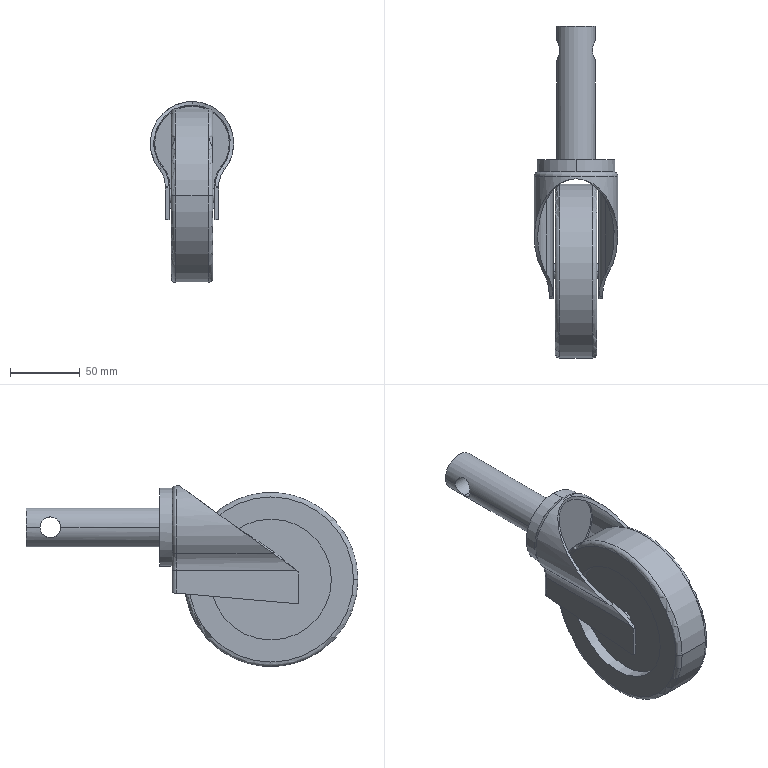Part | NX | features BREP 1 | 1 solid | 66 faces | box 60 x 238.5 x 130 mm | volume 383243 mm3 | cylinder 30 | plane 20 | torus 10 | spline 6 | commonest cylinder face diameters 0.25 x4 10.215 x4 86.9 x4 1.27 x2 6.35 x2 15 x2